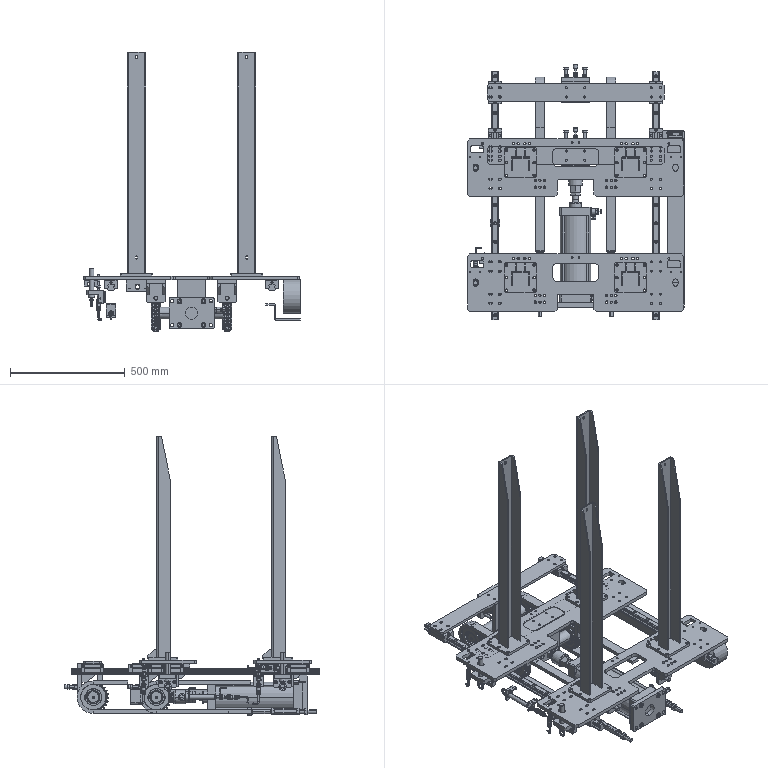Part | SolidWorks | 144 solids | 11348 faces | volume 28618691 mm3 | plane 4864 | cylinder 4431 | cone 1219 | torus 460 | spline 374 | commonest cylinder face diameters 14.66 x416 26.567 x416 20 x364 10.311 x256 9 x232 134 x202